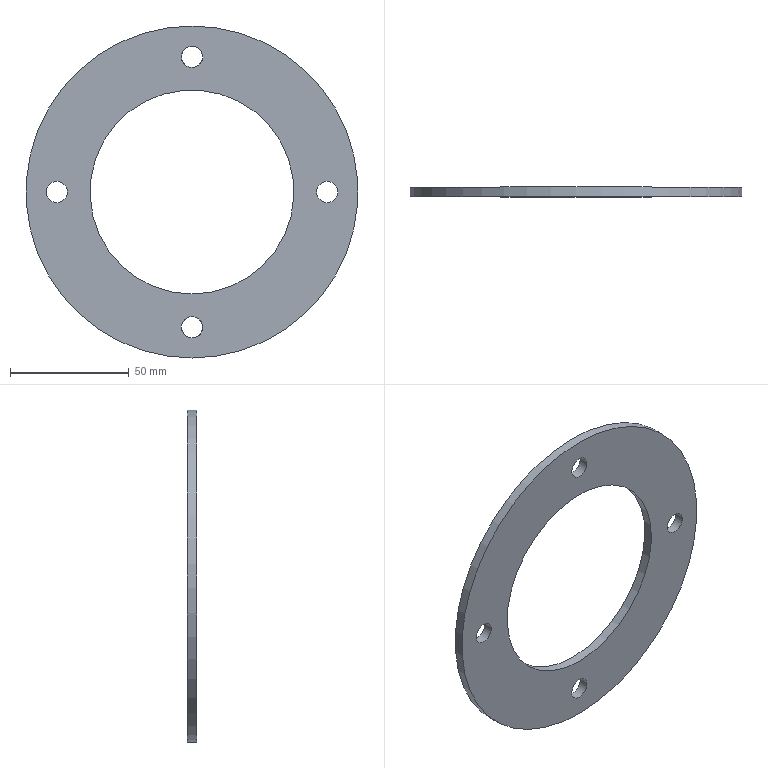Part | NX | features EXTRACT_DATUM_AXIS 8, DATUM_CSYS 6, SKETCH 5, DELETE FACE 4, EXTRACT_DATUM_PLANE 4, EXTRACT_STRING 4, EXTRUDE 4, Instance Feature 3, OFFSET_REGION 3, BREP 1, HOLE PACKAGE 1, Pattern Feature 1, SIMPLE HOLE 1, TRIM BODY 1 | 1 solid | 8 faces | box 140 x 4 x 140 mm | volume 37322 mm3 | cylinder 6 | plane 2 | commonest cylinder face diameters 9 x4 86 x1 140 x1
STEP:
#1=CARTESIAN_POINT('',(0.,-4.,-70.));
#2=VERTEX_POINT('',#1);
#3=CARTESIAN_POINT('',(0.,-4.,0.));
#4=DIRECTION('',(0.,-1.,0.));
#5=DIRECTION('',(0.,0.,-1.));
#6=AXIS2_PLACEMENT_3D('',#3,#4,#5);
#7=CIRCLE('',#6,70.);
#8=EDGE_CURVE('',#2,#2,#7,.T.);
#9=ORIENTED_EDGE('',*,*,#8,.F.);
#10=EDGE_LOOP('',(#9));
#11=FACE_BOUND('',#10,.T.);
#12=CARTESIAN_POINT('',(0.,0.,-70.));
#13=VERTEX_POINT('',#12);
#14=CARTESIAN_POINT('',(0.,0.,0.));
#15=DIRECTION('',(0.,-1.,0.));
#16=DIRECTION('',(0.,0.,-1.));
#17=AXIS2_PLACEMENT_3D('',#14,#15,#16);
#18=CIRCLE('',#17,70.);
#19=EDGE_CURVE('',#13,#13,#18,.T.);
#20=ORIENTED_EDGE('',*,*,#19,.T.);
#21=EDGE_LOOP('',(#20));
#22=FACE_BOUND('',#21,.T.);
#23=CARTESIAN_POINT('',(0.,-10.,0.));
#24=DIRECTION('',(0.,1.,0.));
#25=DIRECTION('',(0.,0.,1.));
#26=AXIS2_PLACEMENT_3D('',#23,#24,#25);
#27=CYLINDRICAL_SURFACE('',#26,70.);
#28=ADVANCED_FACE('',(#11,#22),#27,.T.);
#29=CARTESIAN_POINT('',(-57.,-4.,-4.5));
#30=VERTEX_POINT('',#29);
#31=CARTESIAN_POINT('',(-57.,-4.,0.));
#32=DIRECTION('',(0.,-1.,0.));
#33=DIRECTION('',(0.,0.,-1.));
#34=AXIS2_PLACEMENT_3D('',#31,#32,#33);
#35=CIRCLE('',#34,4.5);
#36=EDGE_CURVE('',#30,#30,#35,.F.);
#37=ORIENTED_EDGE('',*,*,#36,.T.);
#38=EDGE_LOOP('',(#37));
#39=FACE_BOUND('',#38,.T.);
#40=CARTESIAN_POINT('',(0.,-4.,-61.5));
#41=VERTEX_POINT('',#40);
#42=CARTESIAN_POINT('',(0.,-4.,-57.));
#43=DIRECTION('',(0.,-1.,0.));
#44=DIRECTION('',(0.,0.,-1.));
#45=AXIS2_PLACEMENT_3D('',#42,#43,#44);
#46=CIRCLE('',#45,4.5);
#47=EDGE_CURVE('',#41,#41,#46,.F.);
#48=ORIENTED_EDGE('',*,*,#47,.T.);
#49=EDGE_LOOP('',(#48));
#50=FACE_BOUND('',#49,.T.);
#51=CARTESIAN_POINT('',(57.,-4.,-4.5));
#52=VERTEX_POINT('',#51);
#53=CARTESIAN_POINT('',(57.,-4.,0.));
#54=DIRECTION('',(0.,-1.,0.));
#55=DIRECTION('',(0.,0.,-1.));
#56=AXIS2_PLACEMENT_3D('',#53,#54,#55);
#57=CIRCLE('',#56,4.5);
#58=EDGE_CURVE('',#52,#52,#57,.F.);
#59=ORIENTED_EDGE('',*,*,#58,.T.);
#60=EDGE_LOOP('',(#59));
#61=FACE_BOUND('',#60,.T.);
#62=CARTESIAN_POINT('',(0.,-4.,52.5));
#63=VERTEX_POINT('',#62);
#64=CARTESIAN_POINT('',(0.,-4.,57.));
#65=DIRECTION('',(0.,-1.,0.));
#66=DIRECTION('',(0.,0.,-1.));
#67=AXIS2_PLACEMENT_3D('',#64,#65,#66);
#68=CIRCLE('',#67,4.5);
#69=EDGE_CURVE('',#63,#63,#68,.F.);
#70=ORIENTED_EDGE('',*,*,#69,.T.);
#71=EDGE_LOOP('',(#70));
#72=FACE_BOUND('',#71,.T.);
#73=CARTESIAN_POINT('',(0.,-4.,-43.));
#74=VERTEX_POINT('',#73);
#75=CARTESIAN_POINT('',(0.,-4.,0.));
#76=DIRECTION('',(0.,-1.,0.));
#77=DIRECTION('',(0.,0.,-1.));
#78=AXIS2_PLACEMENT_3D('',#75,#76,#77);
#79=CIRCLE('',#78,43.);
#80=EDGE_CURVE('',#74,#74,#79,.T.);
#81=ORIENTED_EDGE('',*,*,#80,.F.);
#82=EDGE_LOOP('',(#81));
#83=FACE_BOUND('',#82,.T.);
#84=ORIENTED_EDGE('',*,*,#8,.T.);
#85=EDGE_LOOP('',(#84));
#86=FACE_BOUND('',#85,.T.);
#87=CARTESIAN_POINT('',(0.,-4.,0.));
#88=DIRECTION('',(0.,-1.,0.));
#89=DIRECTION('',(0.,0.,-1.));
#90=AXIS2_PLACEMENT_3D('',#87,#88,#89);
#91=PLANE('',#90);
#92=ADVANCED_FACE('',(#39,#50,#61,#72,#83,#86),#91,.T.);
#93=CARTESIAN_POINT('',(-57.,0.,4.5));
#94=VERTEX_POINT('',#93);
#95=CARTESIAN_POINT('',(-57.,0.,0.));
#96=DIRECTION('',(0.,-1.,0.));
#97=DIRECTION('',(0.,0.,1.));
#98=AXIS2_PLACEMENT_3D('',#95,#96,#97);
#99=CIRCLE('',#98,4.5);
#100=EDGE_CURVE('',#94,#94,#99,.T.);
#101=ORIENTED_EDGE('',*,*,#100,.T.);
#102=EDGE_LOOP('',(#101));
#103=FACE_BOUND('',#102,.T.);
#104=CARTESIAN_POINT('',(-4.5,0.,-57.));
#105=VERTEX_POINT('',#104);
#106=CARTESIAN_POINT('',(0.,0.,-57.));
#107=DIRECTION('',(0.,-1.,0.));
#108=DIRECTION('',(-1.,0.,0.));
#109=AXIS2_PLACEMENT_3D('',#106,#107,#108);
#110=CIRCLE('',#109,4.5);
#111=EDGE_CURVE('',#105,#105,#110,.T.);
#112=ORIENTED_EDGE('',*,*,#111,.T.);
#113=EDGE_LOOP('',(#112));
#114=FACE_BOUND('',#113,.T.);
#115=CARTESIAN_POINT('',(57.,0.,-4.5));
#116=VERTEX_POINT('',#115);
#117=CARTESIAN_POINT('',(57.,0.,0.));
#118=DIRECTION('',(0.,-1.,0.));
#119=DIRECTION('',(0.,0.,-1.));
#120=AXIS2_PLACEMENT_3D('',#117,#118,#119);
#121=CIRCLE('',#120,4.5);
#122=EDGE_CURVE('',#116,#116,#121,.T.);
#123=ORIENTED_EDGE('',*,*,#122,.T.);
#124=EDGE_LOOP('',(#123));
#125=FACE_BOUND('',#124,.T.);
#126=CARTESIAN_POINT('',(4.5,0.,57.));
#127=VERTEX_POINT('',#126);
#128=CARTESIAN_POINT('',(0.,0.,57.));
#129=DIRECTION('',(0.,-1.,0.));
#130=DIRECTION('',(1.,0.,0.));
#131=AXIS2_PLACEMENT_3D('',#128,#129,#130);
#132=CIRCLE('',#131,4.5);
#133=EDGE_CURVE('',#127,#127,#132,.T.);
#134=ORIENTED_EDGE('',*,*,#133,.T.);
#135=EDGE_LOOP('',(#134));
#136=FACE_BOUND('',#135,.T.);
#137=CARTESIAN_POINT('',(0.,0.,-43.));
#138=VERTEX_POINT('',#137);
#139=CARTESIAN_POINT('',(0.,0.,0.));
#140=DIRECTION('',(0.,-1.,0.));
#141=DIRECTION('',(0.,0.,-1.));
#142=AXIS2_PLACEMENT_3D('',#139,#140,#141);
#143=CIRCLE('',#142,43.);
#144=EDGE_CURVE('',#138,#138,#143,.T.);
#145=ORIENTED_EDGE('',*,*,#144,.T.);
#146=EDGE_LOOP('',(#145));
#147=FACE_BOUND('',#146,.T.);
#148=ORIENTED_EDGE('',*,*,#19,.F.);
#149=EDGE_LOOP('',(#148));
#150=FACE_BOUND('',#149,.T.);
#151=CARTESIAN_POINT('',(0.,0.,0.));
#152=DIRECTION('',(0.,-1.,0.));
#153=DIRECTION('',(0.,0.,-1.));
#154=AXIS2_PLACEMENT_3D('',#151,#152,#153);
#155=PLANE('',#154);
#156=ADVANCED_FACE('',(#103,#114,#125,#136,#147,#150),#155,.F.);
#157=ORIENTED_EDGE('',*,*,#80,.T.);
#158=EDGE_LOOP('',(#157));
#159=FACE_BOUND('',#158,.T.);
#160=ORIENTED_EDGE('',*,*,#144,.F.);
#161=EDGE_LOOP('',(#160));
#162=FACE_BOUND('',#161,.T.);
#163=CARTESIAN_POINT('',(0.,0.,0.));
#164=DIRECTION('',(0.,-1.,0.));
#165=DIRECTION('',(0.,0.,-1.));
#166=AXIS2_PLACEMENT_3D('',#163,#164,#165);
#167=CYLINDRICAL_SURFACE('',#166,43.);
#168=ADVANCED_FACE('',(#159,#162),#167,.F.);
#169=ORIENTED_EDGE('',*,*,#69,.F.);
#170=EDGE_LOOP('',(#169));
#171=FACE_BOUND('',#170,.T.);
#172=ORIENTED_EDGE('',*,*,#133,.F.);
#173=EDGE_LOOP('',(#172));
#174=FACE_BOUND('',#173,.T.);
#175=CARTESIAN_POINT('',(0.,-6.,57.));
#176=DIRECTION('',(0.,1.,0.));
#177=DIRECTION('',(0.,0.,1.));
#178=AXIS2_PLACEMENT_3D('',#175,#176,#177);
#179=CYLINDRICAL_SURFACE('',#178,4.5);
#180=ADVANCED_FACE('',(#171,#174),#179,.F.);
#181=ORIENTED_EDGE('',*,*,#58,.F.);
#182=EDGE_LOOP('',(#181));
#183=FACE_BOUND('',#182,.T.);
#184=ORIENTED_EDGE('',*,*,#122,.F.);
#185=EDGE_LOOP('',(#184));
#186=FACE_BOUND('',#185,.T.);
#187=CARTESIAN_POINT('',(57.,-6.,0.));
#188=DIRECTION('',(0.,1.,0.));
#189=DIRECTION('',(0.,0.,1.));
#190=AXIS2_PLACEMENT_3D('',#187,#188,#189);
#191=CYLINDRICAL_SURFACE('',#190,4.5);
#192=ADVANCED_FACE('',(#183,#186),#191,.F.);
#193=ORIENTED_EDGE('',*,*,#47,.F.);
#194=EDGE_LOOP('',(#193));
#195=FACE_BOUND('',#194,.T.);
#196=ORIENTED_EDGE('',*,*,#111,.F.);
#197=EDGE_LOOP('',(#196));
#198=FACE_BOUND('',#197,.T.);
#199=CARTESIAN_POINT('',(0.,-6.,-57.));
#200=DIRECTION('',(0.,1.,0.));
#201=DIRECTION('',(0.,0.,1.));
#202=AXIS2_PLACEMENT_3D('',#199,#200,#201);
#203=CYLINDRICAL_SURFACE('',#202,4.5);
#204=ADVANCED_FACE('',(#195,#198),#203,.F.);
#205=ORIENTED_EDGE('',*,*,#36,.F.);
#206=EDGE_LOOP('',(#205));
#207=FACE_BOUND('',#206,.T.);
#208=ORIENTED_EDGE('',*,*,#100,.F.);
#209=EDGE_LOOP('',(#208));
#210=FACE_BOUND('',#209,.T.);
#211=CARTESIAN_POINT('',(-57.,-6.,0.));
#212=DIRECTION('',(0.,1.,0.));
#213=DIRECTION('',(0.,0.,1.));
#214=AXIS2_PLACEMENT_3D('',#211,#212,#213);
#215=CYLINDRICAL_SURFACE('',#214,4.5);
#216=ADVANCED_FACE('',(#207,#210),#215,.F.);
#217=CLOSED_SHELL('',(#28,#92,#156,#168,#180,#192,#204,#216));
#218=MANIFOLD_SOLID_BREP('',#217);
#219=(LENGTH_UNIT()NAMED_UNIT(*)SI_UNIT(.MILLI.,.METRE.));
#220=UNCERTAINTY_MEASURE_WITH_UNIT(LENGTH_MEASURE(0.00001),#219,'','');
#221=(NAMED_UNIT(*)PLANE_ANGLE_UNIT()SI_UNIT($,.RADIAN.));
#222=(NAMED_UNIT(*)SI_UNIT($,.STERADIAN.)SOLID_ANGLE_UNIT());
#223=(GEOMETRIC_REPRESENTATION_CONTEXT(3)GLOBAL_UNCERTAINTY_ASSIGNED_CONTEXT((#220))GLOBAL_UNIT_ASSIGNED_CONTEXT((#219,#221,#222))REPRESENTATION_CONTEXT('',''));
#224=ADVANCED_BREP_SHAPE_REPRESENTATION('',(#218),#223);